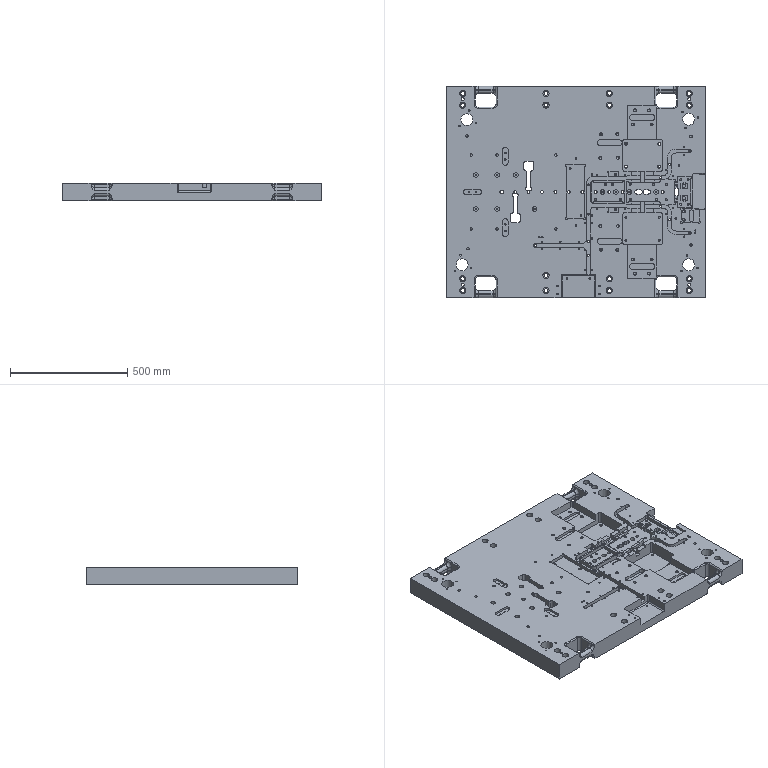Part | STEP file | 1_id94_x_t | 1 solid | 878 faces | box 1100 x 900 x 75 mm | volume 64161476 mm3 | cylinder 417 | plane 260 | cone 151 | torus 48 | sphere 2 | commonest cylinder face diameters 10 x66 25.4 x48 10.716 x32 5.105 x30 6.528 x18 7 x18